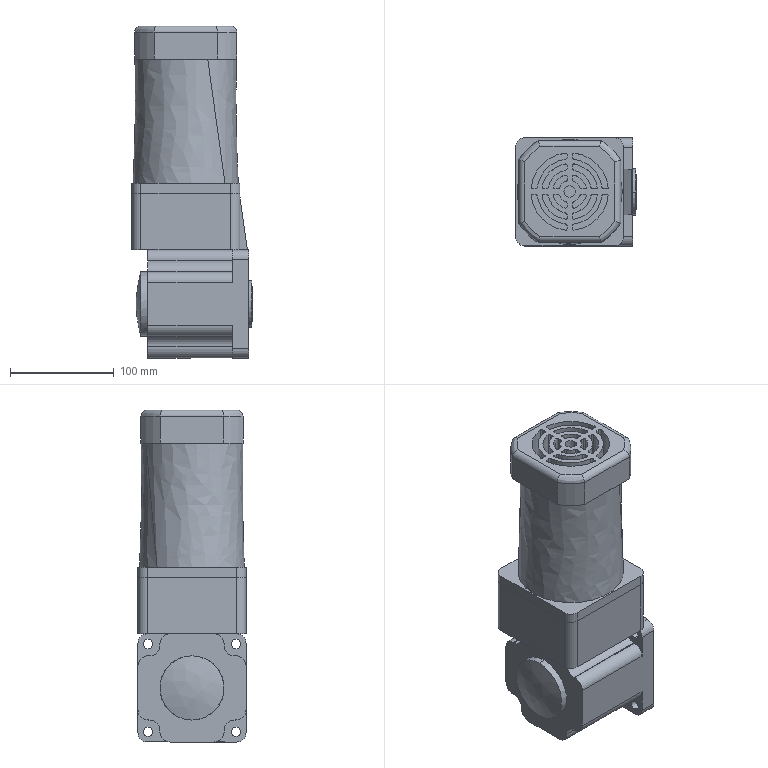Part | STEP file | 200W right-angle motor | 3 solids | 254 faces | box 116.75 x 104.5 x 320.75 mm | volume 2722546 mm3 | cylinder 150 | plane 95 | spline 7 | cone 2 | commonest cylinder face diameters 3 x30 4 x24 20 x16 18 x12 2 x8 9 x8